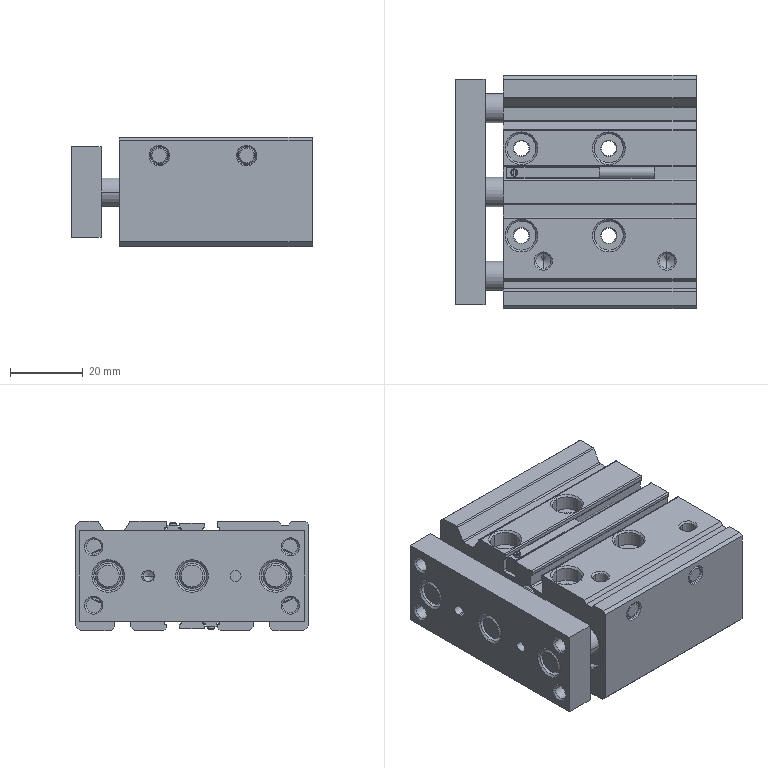Part | SolidWorks | features BaseBody 4 | 4 solids | 453 faces | box 66 x 64 x 30 mm | volume 89467 mm3 | cylinder 185 | plane 156 | cone 110 | spline 2 | commonest cylinder face diameters 4.134 x28 8 x26 3 x25 0.4 x20 0.8 x20 0.6 x10